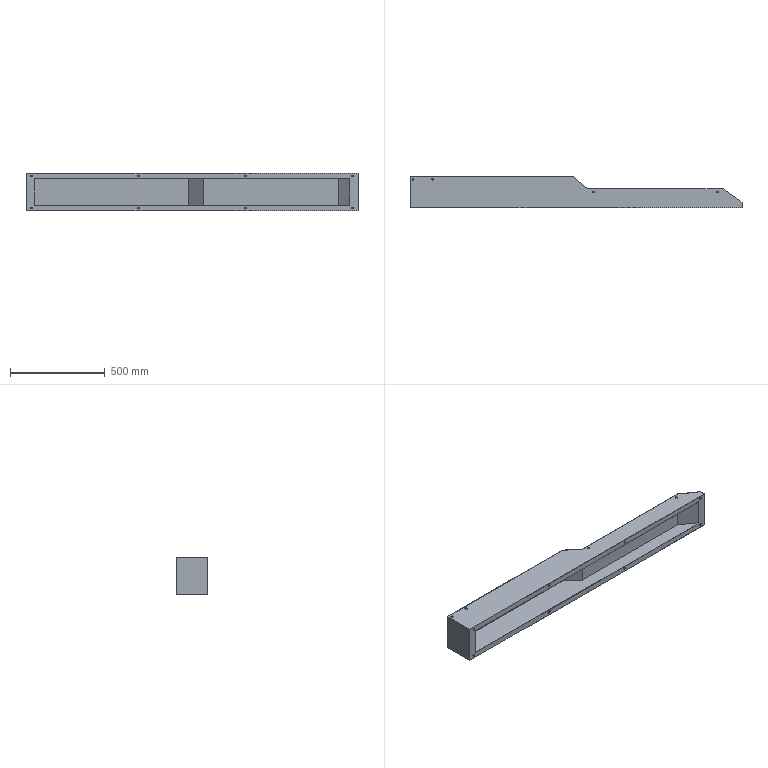Part | SolidWorks | features ICE 5, HoleWzd 2, Extrusion 1, Shell 1 | 1 solid | 166 faces | box 1750 x 167 x 200 mm | volume 1937226 mm3 | plane 118 | cylinder 48 | commonest cylinder face diameters 6.8 x24 9 x24